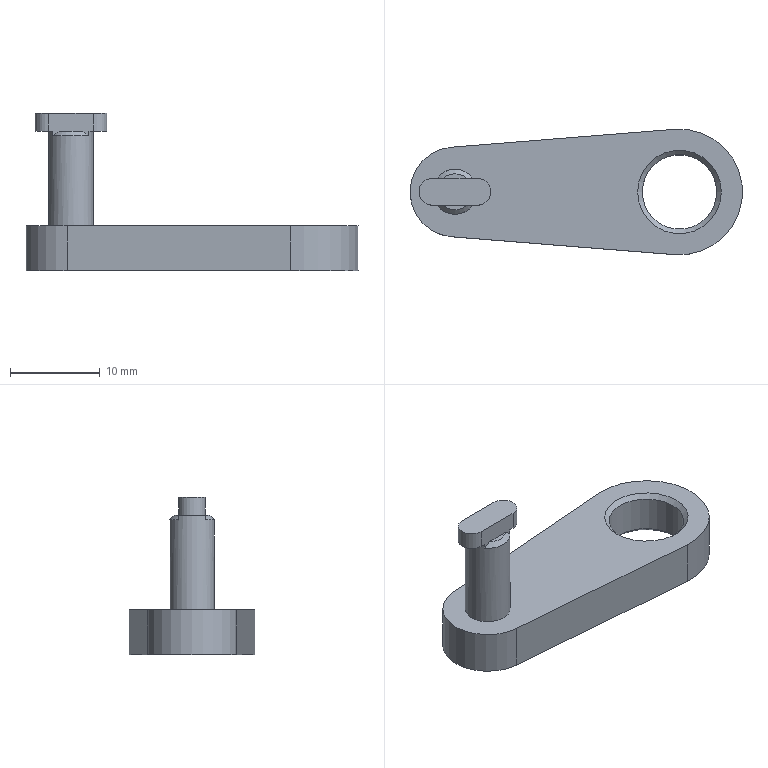Part | NX | features BREP 1 | 1 solid | 21 faces | box 37 x 14 x 17.5 mm | volume 2058 mm3 | plane 11 | cylinder 6 | cone 4 | commonest cylinder face diameters 3 x2 5 x1 8.3 x1 10 x1 14 x1
STEP:
#1=CARTESIAN_POINT('',(4.65,0.,2.5));
#2=VERTEX_POINT('',#1);
#3=CARTESIAN_POINT('',(0.,0.,2.5));
#4=DIRECTION('',(0.,0.,-1.));
#5=DIRECTION('',(1.,0.,0.));
#6=AXIS2_PLACEMENT_3D('',#3,#4,#5);
#7=CIRCLE('',#6,4.65);
#8=EDGE_CURVE('',#2,#2,#7,.T.);
#9=ORIENTED_EDGE('',*,*,#8,.F.);
#10=EDGE_LOOP('',(#9));
#11=FACE_BOUND('',#10,.T.);
#12=CARTESIAN_POINT('',(4.15,0.,2.));
#13=VERTEX_POINT('',#12);
#14=CARTESIAN_POINT('',(0.,0.,2.));
#15=DIRECTION('',(0.,0.,1.));
#16=DIRECTION('',(1.,0.,0.));
#17=AXIS2_PLACEMENT_3D('',#14,#15,#16);
#18=CIRCLE('',#17,4.15);
#19=EDGE_CURVE('',#13,#13,#18,.T.);
#20=ORIENTED_EDGE('',*,*,#19,.F.);
#21=EDGE_LOOP('',(#20));
#22=FACE_BOUND('',#21,.T.);
#23=CARTESIAN_POINT('',(0.,0.,2.));
#24=DIRECTION('',(0.,0.,1.));
#25=DIRECTION('',(-1.,0.,0.));
#26=AXIS2_PLACEMENT_3D('',#23,#24,#25);
#27=CONICAL_SURFACE('',#26,4.15,0.7854);
#28=ADVANCED_FACE('',(#11,#22),#27,.F.);
#29=CARTESIAN_POINT('',(4.65,0.,-2.5));
#30=VERTEX_POINT('',#29);
#31=CARTESIAN_POINT('',(0.,0.,-2.5));
#32=DIRECTION('',(0.,0.,1.));
#33=DIRECTION('',(1.,0.,0.));
#34=AXIS2_PLACEMENT_3D('',#31,#32,#33);
#35=CIRCLE('',#34,4.65);
#36=EDGE_CURVE('',#30,#30,#35,.T.);
#37=ORIENTED_EDGE('',*,*,#36,.F.);
#38=EDGE_LOOP('',(#37));
#39=FACE_BOUND('',#38,.T.);
#40=CARTESIAN_POINT('',(4.15,0.,-2.));
#41=VERTEX_POINT('',#40);
#42=CARTESIAN_POINT('',(0.,0.,-2.));
#43=DIRECTION('',(0.,0.,-1.));
#44=DIRECTION('',(1.,0.,0.));
#45=AXIS2_PLACEMENT_3D('',#42,#43,#44);
#46=CIRCLE('',#45,4.15);
#47=EDGE_CURVE('',#41,#41,#46,.T.);
#48=ORIENTED_EDGE('',*,*,#47,.F.);
#49=EDGE_LOOP('',(#48));
#50=FACE_BOUND('',#49,.T.);
#51=CARTESIAN_POINT('',(0.,0.,-2.5));
#52=DIRECTION('',(0.,0.,-1.));
#53=DIRECTION('',(1.,0.,0.));
#54=AXIS2_PLACEMENT_3D('',#51,#52,#53);
#55=CONICAL_SURFACE('',#54,4.65,0.7854);
#56=ADVANCED_FACE('',(#39,#50),#55,.F.);
#57=ORIENTED_EDGE('',*,*,#19,.T.);
#58=EDGE_LOOP('',(#57));
#59=FACE_BOUND('',#58,.T.);
#60=ORIENTED_EDGE('',*,*,#47,.T.);
#61=EDGE_LOOP('',(#60));
#62=FACE_BOUND('',#61,.T.);
#63=CARTESIAN_POINT('',(0.,0.,-2.5));
#64=DIRECTION('',(0.,0.,1.));
#65=DIRECTION('',(-1.,0.,0.));
#66=AXIS2_PLACEMENT_3D('',#63,#64,#65);
#67=CYLINDRICAL_SURFACE('',#66,4.15);
#68=ADVANCED_FACE('',(#59,#62),#67,.F.);
#69=CARTESIAN_POINT('',(-27.5,1.5,15.));
#70=VERTEX_POINT('',#69);
#71=CARTESIAN_POINT('',(-27.5,-1.5,15.));
#72=VERTEX_POINT('',#71);
#73=CARTESIAN_POINT('',(-27.5,0.,15.));
#74=DIRECTION('',(0.,0.,1.));
#75=DIRECTION('',(1.,0.,0.));
#76=AXIS2_PLACEMENT_3D('',#73,#74,#75);
#77=CIRCLE('',#76,1.5);
#78=EDGE_CURVE('',#70,#72,#77,.T.);
#79=ORIENTED_EDGE('',*,*,#78,.F.);
#80=CARTESIAN_POINT('',(-27.5,1.5,13.));
#81=VERTEX_POINT('',#80);
#82=CARTESIAN_POINT('',(-27.5,1.5,15.));
#83=DIRECTION('',(0.,0.,-1.));
#84=VECTOR('',#83,1000.);
#85=LINE('',#82,#84);
#86=EDGE_CURVE('',#70,#81,#85,.T.);
#87=ORIENTED_EDGE('',*,*,#86,.T.);
#88=CARTESIAN_POINT('',(-27.5,-1.5,13.));
#89=VERTEX_POINT('',#88);
#90=CARTESIAN_POINT('',(-27.5,0.,13.));
#91=DIRECTION('',(0.,0.,1.));
#92=DIRECTION('',(1.,0.,0.));
#93=AXIS2_PLACEMENT_3D('',#90,#91,#92);
#94=CIRCLE('',#93,1.5);
#95=EDGE_CURVE('',#81,#89,#94,.T.);
#96=ORIENTED_EDGE('',*,*,#95,.T.);
#97=CARTESIAN_POINT('',(-27.5,-1.5,15.));
#98=DIRECTION('',(0.,0.,-1.));
#99=VECTOR('',#98,1000.);
#100=LINE('',#97,#99);
#101=EDGE_CURVE('',#72,#89,#100,.T.);
#102=ORIENTED_EDGE('',*,*,#101,.F.);
#103=EDGE_LOOP('',(#79,#87,#96,#102));
#104=FACE_BOUND('',#103,.T.);
#105=CARTESIAN_POINT('',(-27.5,0.,15.));
#106=DIRECTION('',(0.,0.,-1.));
#107=DIRECTION('',(1.,0.,0.));
#108=AXIS2_PLACEMENT_3D('',#105,#106,#107);
#109=CYLINDRICAL_SURFACE('',#108,1.5);
#110=ADVANCED_FACE('',(#104),#109,.T.);
#111=CARTESIAN_POINT('',(-22.5,0.,2.5));
#112=VERTEX_POINT('',#111);
#113=CARTESIAN_POINT('',(-25.,0.,2.5));
#114=DIRECTION('',(0.,0.,1.));
#115=DIRECTION('',(1.,0.,0.));
#116=AXIS2_PLACEMENT_3D('',#113,#114,#115);
#117=CIRCLE('',#116,2.5);
#118=EDGE_CURVE('',#112,#112,#117,.T.);
#119=ORIENTED_EDGE('',*,*,#118,.T.);
#120=EDGE_LOOP('',(#119));
#121=FACE_BOUND('',#120,.T.);
#122=CARTESIAN_POINT('',(-23.,-1.5,13.));
#123=VERTEX_POINT('',#122);
#124=CARTESIAN_POINT('',(-23.,1.5,13.));
#125=VERTEX_POINT('',#124);
#126=CARTESIAN_POINT('',(-25.,0.,13.));
#127=DIRECTION('',(0.,0.,1.));
#128=DIRECTION('',(1.,0.,0.));
#129=AXIS2_PLACEMENT_3D('',#126,#127,#128);
#130=CIRCLE('',#129,2.5);
#131=EDGE_CURVE('',#123,#125,#130,.T.);
#132=ORIENTED_EDGE('',*,*,#131,.F.);
#133=CARTESIAN_POINT('',(-23.,-1.5,12.5));
#134=VERTEX_POINT('',#133);
#135=CARTESIAN_POINT('',(-23.,-1.5,13.));
#136=DIRECTION('',(0.,0.,-1.));
#137=VECTOR('',#136,1000.);
#138=LINE('',#135,#137);
#139=EDGE_CURVE('',#123,#134,#138,.T.);
#140=ORIENTED_EDGE('',*,*,#139,.T.);
#141=CARTESIAN_POINT('',(-27.,-1.5,12.5));
#142=VERTEX_POINT('',#141);
#143=CARTESIAN_POINT('',(-25.,0.,12.5));
#144=DIRECTION('',(0.,0.,-1.));
#145=DIRECTION('',(1.,0.,0.));
#146=AXIS2_PLACEMENT_3D('',#143,#144,#145);
#147=CIRCLE('',#146,2.5);
#148=EDGE_CURVE('',#134,#142,#147,.T.);
#149=ORIENTED_EDGE('',*,*,#148,.T.);
#150=CARTESIAN_POINT('',(-27.,-1.5,13.));
#151=VERTEX_POINT('',#150);
#152=CARTESIAN_POINT('',(-27.,-1.5,12.5));
#153=DIRECTION('',(0.,0.,1.));
#154=VECTOR('',#153,1000.);
#155=LINE('',#152,#154);
#156=EDGE_CURVE('',#142,#151,#155,.T.);
#157=ORIENTED_EDGE('',*,*,#156,.T.);
#158=CARTESIAN_POINT('',(-27.,1.5,13.));
#159=VERTEX_POINT('',#158);
#160=CARTESIAN_POINT('',(-25.,0.,13.));
#161=DIRECTION('',(0.,0.,1.));
#162=DIRECTION('',(1.,0.,0.));
#163=AXIS2_PLACEMENT_3D('',#160,#161,#162);
#164=CIRCLE('',#163,2.5);
#165=EDGE_CURVE('',#159,#151,#164,.T.);
#166=ORIENTED_EDGE('',*,*,#165,.F.);
#167=CARTESIAN_POINT('',(-27.,1.5,12.5));
#168=VERTEX_POINT('',#167);
#169=CARTESIAN_POINT('',(-27.,1.5,13.));
#170=DIRECTION('',(0.,0.,-1.));
#171=VECTOR('',#170,1000.);
#172=LINE('',#169,#171);
#173=EDGE_CURVE('',#159,#168,#172,.T.);
#174=ORIENTED_EDGE('',*,*,#173,.T.);
#175=CARTESIAN_POINT('',(-23.,1.5,12.5));
#176=VERTEX_POINT('',#175);
#177=CARTESIAN_POINT('',(-25.,0.,12.5));
#178=DIRECTION('',(0.,0.,-1.));
#179=DIRECTION('',(1.,0.,0.));
#180=AXIS2_PLACEMENT_3D('',#177,#178,#179);
#181=CIRCLE('',#180,2.5);
#182=EDGE_CURVE('',#168,#176,#181,.T.);
#183=ORIENTED_EDGE('',*,*,#182,.T.);
#184=CARTESIAN_POINT('',(-23.,1.5,12.5));
#185=DIRECTION('',(0.,0.,1.));
#186=VECTOR('',#185,1000.);
#187=LINE('',#184,#186);
#188=EDGE_CURVE('',#176,#125,#187,.T.);
#189=ORIENTED_EDGE('',*,*,#188,.T.);
#190=EDGE_LOOP('',(#132,#140,#149,#157,#166,#174,#183,#189));
#191=FACE_BOUND('',#190,.T.);
#192=CARTESIAN_POINT('',(-25.,0.,13.));
#193=DIRECTION('',(0.,0.,-1.));
#194=DIRECTION('',(1.,0.,0.));
#195=AXIS2_PLACEMENT_3D('',#192,#193,#194);
#196=CYLINDRICAL_SURFACE('',#195,2.5);
#197=ADVANCED_FACE('',(#121,#191),#196,.T.);
#198=CARTESIAN_POINT('',(-25.4,4.984,2.5));
#199=VERTEX_POINT('',#198);
#200=CARTESIAN_POINT('',(-25.4,-4.984,2.5));
#201=VERTEX_POINT('',#200);
#202=CARTESIAN_POINT('',(-25.,0.,2.5));
#203=DIRECTION('',(0.,0.,1.));
#204=DIRECTION('',(1.,0.,0.));
#205=AXIS2_PLACEMENT_3D('',#202,#203,#204);
#206=CIRCLE('',#205,5.);
#207=EDGE_CURVE('',#199,#201,#206,.T.);
#208=ORIENTED_EDGE('',*,*,#207,.F.);
#209=CARTESIAN_POINT('',(-25.4,4.984,-2.5));
#210=VERTEX_POINT('',#209);
#211=CARTESIAN_POINT('',(-25.4,4.984,2.5));
#212=DIRECTION('',(0.,0.,-1.));
#213=VECTOR('',#212,1000.);
#214=LINE('',#211,#213);
#215=EDGE_CURVE('',#199,#210,#214,.T.);
#216=ORIENTED_EDGE('',*,*,#215,.T.);
#217=CARTESIAN_POINT('',(-25.4,-4.984,-2.5));
#218=VERTEX_POINT('',#217);
#219=CARTESIAN_POINT('',(-25.,0.,-2.5));
#220=DIRECTION('',(0.,0.,1.));
#221=DIRECTION('',(1.,0.,0.));
#222=AXIS2_PLACEMENT_3D('',#219,#220,#221);
#223=CIRCLE('',#222,5.);
#224=EDGE_CURVE('',#210,#218,#223,.T.);
#225=ORIENTED_EDGE('',*,*,#224,.T.);
#226=CARTESIAN_POINT('',(-25.4,-4.984,2.5));
#227=DIRECTION('',(0.,0.,-1.));
#228=VECTOR('',#227,1000.);
#229=LINE('',#226,#228);
#230=EDGE_CURVE('',#201,#218,#229,.T.);
#231=ORIENTED_EDGE('',*,*,#230,.F.);
#232=EDGE_LOOP('',(#208,#216,#225,#231));
#233=FACE_BOUND('',#232,.T.);
#234=CARTESIAN_POINT('',(-25.,0.,2.5));
#235=DIRECTION('',(0.,0.,-1.));
#236=DIRECTION('',(1.,0.,0.));
#237=AXIS2_PLACEMENT_3D('',#234,#235,#236);
#238=CYLINDRICAL_SURFACE('',#237,5.);
#239=ADVANCED_FACE('',(#233),#238,.T.);
#240=CARTESIAN_POINT('',(-23.677,1.5,13.));
#241=VERTEX_POINT('',#240);
#242=CARTESIAN_POINT('',(-26.323,1.5,13.));
#243=VERTEX_POINT('',#242);
#244=CARTESIAN_POINT('',(-27.5,1.5,13.));
#245=DIRECTION('',(-1.,0.,0.));
#246=VECTOR('',#245,1000.);
#247=LINE('',#244,#246);
#248=EDGE_CURVE('',#241,#243,#247,.T.);
#249=ORIENTED_EDGE('',*,*,#248,.F.);
#250=CARTESIAN_POINT('',(-25.,0.,13.));
#251=DIRECTION('',(0.,0.,1.));
#252=DIRECTION('',(1.,0.,0.));
#253=AXIS2_PLACEMENT_3D('',#250,#251,#252);
#254=CIRCLE('',#253,2.);
#255=EDGE_CURVE('',#241,#243,#254,.T.);
#256=ORIENTED_EDGE('',*,*,#255,.T.);
#257=EDGE_LOOP('',(#249,#256));
#258=FACE_BOUND('',#257,.T.);
#259=CARTESIAN_POINT('',(-25.,0.,13.));
#260=DIRECTION('',(0.,0.,1.));
#261=DIRECTION('',(-1.,0.,0.));
#262=AXIS2_PLACEMENT_3D('',#259,#260,#261);
#263=PLANE('',#262);
#264=ADVANCED_FACE('',(#258),#263,.T.);
#265=ORIENTED_EDGE('',*,*,#8,.T.);
#266=EDGE_LOOP('',(#265));
#267=FACE_BOUND('',#266,.T.);
#268=CARTESIAN_POINT('',(-0.56,6.978,2.5));
#269=VERTEX_POINT('',#268);
#270=CARTESIAN_POINT('',(-25.4,4.984,2.5));
#271=DIRECTION('',(-0.9968,-0.08,0.));
#272=VECTOR('',#271,1000.);
#273=LINE('',#270,#272);
#274=EDGE_CURVE('',#269,#199,#273,.T.);
#275=ORIENTED_EDGE('',*,*,#274,.T.);
#276=ORIENTED_EDGE('',*,*,#207,.T.);
#277=CARTESIAN_POINT('',(-0.56,-6.978,2.5));
#278=VERTEX_POINT('',#277);
#279=CARTESIAN_POINT('',(-0.56,-6.978,2.5));
#280=DIRECTION('',(0.9968,-0.08,0.));
#281=VECTOR('',#280,1000.);
#282=LINE('',#279,#281);
#283=EDGE_CURVE('',#201,#278,#282,.T.);
#284=ORIENTED_EDGE('',*,*,#283,.T.);
#285=CARTESIAN_POINT('',(0.,0.,2.5));
#286=DIRECTION('',(0.,0.,1.));
#287=DIRECTION('',(1.,0.,0.));
#288=AXIS2_PLACEMENT_3D('',#285,#286,#287);
#289=CIRCLE('',#288,7.);
#290=EDGE_CURVE('',#278,#269,#289,.T.);
#291=ORIENTED_EDGE('',*,*,#290,.T.);
#292=EDGE_LOOP('',(#275,#276,#284,#291));
#293=FACE_BOUND('',#292,.T.);
#294=ORIENTED_EDGE('',*,*,#118,.F.);
#295=EDGE_LOOP('',(#294));
#296=FACE_BOUND('',#295,.T.);
#297=CARTESIAN_POINT('',(-25.,0.,2.5));
#298=DIRECTION('',(0.,0.,1.));
#299=DIRECTION('',(-1.,0.,0.));
#300=AXIS2_PLACEMENT_3D('',#297,#298,#299);
#301=PLANE('',#300);
#302=ADVANCED_FACE('',(#267,#293,#296),#301,.T.);
#303=CARTESIAN_POINT('',(-0.56,-6.978,-2.5));
#304=VERTEX_POINT('',#303);
#305=CARTESIAN_POINT('',(-0.56,-6.978,-2.5));
#306=DIRECTION('',(0.9968,-0.08,0.));
#307=VECTOR('',#306,1000.);
#308=LINE('',#305,#307);
#309=EDGE_CURVE('',#218,#304,#308,.T.);
#310=ORIENTED_EDGE('',*,*,#309,.T.);
#311=CARTESIAN_POINT('',(-0.56,-6.978,2.5));
#312=DIRECTION('',(0.,0.,-1.));
#313=VECTOR('',#312,1000.);
#314=LINE('',#311,#313);
#315=EDGE_CURVE('',#278,#304,#314,.T.);
#316=ORIENTED_EDGE('',*,*,#315,.F.);
#317=ORIENTED_EDGE('',*,*,#283,.F.);
#318=ORIENTED_EDGE('',*,*,#230,.T.);
#319=EDGE_LOOP('',(#310,#316,#317,#318));
#320=FACE_BOUND('',#319,.T.);
#321=CARTESIAN_POINT('',(-0.56,-6.978,2.5));
#322=DIRECTION('',(0.08,0.9968,0.));
#323=DIRECTION('',(0.9968,-0.08,0.));
#324=AXIS2_PLACEMENT_3D('',#321,#322,#323);
#325=PLANE('',#324);
#326=ADVANCED_FACE('',(#320),#325,.F.);
#327=CARTESIAN_POINT('',(-0.56,6.978,-2.5));
#328=VERTEX_POINT('',#327);
#329=CARTESIAN_POINT('',(0.,0.,-2.5));
#330=DIRECTION('',(0.,0.,1.));
#331=DIRECTION('',(1.,0.,0.));
#332=AXIS2_PLACEMENT_3D('',#329,#330,#331);
#333=CIRCLE('',#332,7.);
#334=EDGE_CURVE('',#304,#328,#333,.T.);
#335=ORIENTED_EDGE('',*,*,#334,.T.);
#336=CARTESIAN_POINT('',(-0.56,6.978,2.5));
#337=DIRECTION('',(0.,0.,-1.));
#338=VECTOR('',#337,1000.);
#339=LINE('',#336,#338);
#340=EDGE_CURVE('',#269,#328,#339,.T.);
#341=ORIENTED_EDGE('',*,*,#340,.F.);
#342=ORIENTED_EDGE('',*,*,#290,.F.);
#343=ORIENTED_EDGE('',*,*,#315,.T.);
#344=EDGE_LOOP('',(#335,#341,#342,#343));
#345=FACE_BOUND('',#344,.T.);
#346=CARTESIAN_POINT('',(0.,0.,2.5));
#347=DIRECTION('',(0.,0.,-1.));
#348=DIRECTION('',(1.,0.,0.));
#349=AXIS2_PLACEMENT_3D('',#346,#347,#348);
#350=CYLINDRICAL_SURFACE('',#349,7.);
#351=ADVANCED_FACE('',(#345),#350,.T.);
#352=CARTESIAN_POINT('',(-25.4,4.984,-2.5));
#353=DIRECTION('',(-0.9968,-0.08,0.));
#354=VECTOR('',#353,1000.);
#355=LINE('',#352,#354);
#356=EDGE_CURVE('',#328,#210,#355,.T.);
#357=ORIENTED_EDGE('',*,*,#356,.T.);
#358=ORIENTED_EDGE('',*,*,#215,.F.);
#359=ORIENTED_EDGE('',*,*,#274,.F.);
#360=ORIENTED_EDGE('',*,*,#340,.T.);
#361=EDGE_LOOP('',(#357,#358,#359,#360));
#362=FACE_BOUND('',#361,.T.);
#363=CARTESIAN_POINT('',(-25.4,4.984,2.5));
#364=DIRECTION('',(0.08,-0.9968,0.));
#365=DIRECTION('',(-0.9968,-0.08,0.));
#366=AXIS2_PLACEMENT_3D('',#363,#364,#365);
#367=PLANE('',#366);
#368=ADVANCED_FACE('',(#362),#367,.F.);
#369=ORIENTED_EDGE('',*,*,#36,.T.);
#370=EDGE_LOOP('',(#369));
#371=FACE_BOUND('',#370,.T.);
#372=ORIENTED_EDGE('',*,*,#224,.F.);
#373=ORIENTED_EDGE('',*,*,#356,.F.);
#374=ORIENTED_EDGE('',*,*,#334,.F.);
#375=ORIENTED_EDGE('',*,*,#309,.F.);
#376=EDGE_LOOP('',(#372,#373,#374,#375));
#377=FACE_BOUND('',#376,.T.);
#378=CARTESIAN_POINT('',(-25.,0.,-2.5));
#379=DIRECTION('',(0.,0.,1.));
#380=DIRECTION('',(-1.,0.,0.));
#381=AXIS2_PLACEMENT_3D('',#378,#379,#380);
#382=PLANE('',#381);
#383=ADVANCED_FACE('',(#371,#377),#382,.F.);
#384=CARTESIAN_POINT('',(-26.323,-1.5,13.));
#385=VERTEX_POINT('',#384);
#386=CARTESIAN_POINT('',(-23.677,-1.5,13.));
#387=VERTEX_POINT('',#386);
#388=CARTESIAN_POINT('',(-27.5,-1.5,13.));
#389=DIRECTION('',(1.,0.,0.));
#390=VECTOR('',#389,1000.);
#391=LINE('',#388,#390);
#392=EDGE_CURVE('',#385,#387,#391,.T.);
#393=ORIENTED_EDGE('',*,*,#392,.F.);
#394=CARTESIAN_POINT('',(-25.,0.,13.));
#395=DIRECTION('',(0.,0.,1.));
#396=DIRECTION('',(1.,0.,0.));
#397=AXIS2_PLACEMENT_3D('',#394,#395,#396);
#398=CIRCLE('',#397,2.);
#399=EDGE_CURVE('',#385,#387,#398,.T.);
#400=ORIENTED_EDGE('',*,*,#399,.T.);
#401=EDGE_LOOP('',(#393,#400));
#402=FACE_BOUND('',#401,.T.);
#403=CARTESIAN_POINT('',(-25.,0.,13.));
#404=DIRECTION('',(0.,0.,1.));
#405=DIRECTION('',(-1.,0.,0.));
#406=AXIS2_PLACEMENT_3D('',#403,#404,#405);
#407=PLANE('',#406);
#408=ADVANCED_FACE('',(#402),#407,.T.);
#409=CARTESIAN_POINT('',(-27.5,1.5,13.));
#410=DIRECTION('',(-1.,0.,0.));
#411=VECTOR('',#410,1000.);
#412=LINE('',#409,#411);
#413=EDGE_CURVE('',#159,#81,#412,.T.);
#414=ORIENTED_EDGE('',*,*,#413,.F.);
#415=ORIENTED_EDGE('',*,*,#165,.T.);
#416=CARTESIAN_POINT('',(-27.5,-1.5,13.));
#417=DIRECTION('',(1.,0.,0.));
#418=VECTOR('',#417,1000.);
#419=LINE('',#416,#418);
#420=EDGE_CURVE('',#89,#151,#419,.T.);
#421=ORIENTED_EDGE('',*,*,#420,.F.);
#422=ORIENTED_EDGE('',*,*,#95,.F.);
#423=EDGE_LOOP('',(#414,#415,#421,#422));
#424=FACE_BOUND('',#423,.T.);
#425=CARTESIAN_POINT('',(-27.5,0.,13.));
#426=DIRECTION('',(0.,0.,1.));
#427=DIRECTION('',(-1.,0.,0.));
#428=AXIS2_PLACEMENT_3D('',#425,#426,#427);
#429=PLANE('',#428);
#430=ADVANCED_FACE('',(#424),#429,.F.);
#431=CARTESIAN_POINT('',(-22.5,-1.5,13.));
#432=VERTEX_POINT('',#431);
#433=CARTESIAN_POINT('',(-27.5,-1.5,13.));
#434=DIRECTION('',(1.,0.,0.));
#435=VECTOR('',#434,1000.);
#436=LINE('',#433,#435);
#437=EDGE_CURVE('',#123,#432,#436,.T.);
#438=ORIENTED_EDGE('',*,*,#437,.F.);
#439=ORIENTED_EDGE('',*,*,#131,.T.);
#440=CARTESIAN_POINT('',(-22.5,1.5,13.));
#441=VERTEX_POINT('',#440);
#442=CARTESIAN_POINT('',(-27.5,1.5,13.));
#443=DIRECTION('',(-1.,0.,0.));
#444=VECTOR('',#443,1000.);
#445=LINE('',#442,#444);
#446=EDGE_CURVE('',#441,#125,#445,.T.);
#447=ORIENTED_EDGE('',*,*,#446,.F.);
#448=CARTESIAN_POINT('',(-22.5,0.,13.));
#449=DIRECTION('',(0.,0.,1.));
#450=DIRECTION('',(1.,0.,0.));
#451=AXIS2_PLACEMENT_3D('',#448,#449,#450);
#452=CIRCLE('',#451,1.5);
#453=EDGE_CURVE('',#432,#441,#452,.T.);
#454=ORIENTED_EDGE('',*,*,#453,.F.);
#455=EDGE_LOOP('',(#438,#439,#447,#454));
#456=FACE_BOUND('',#455,.T.);
#457=CARTESIAN_POINT('',(-27.5,0.,13.));
#458=DIRECTION('',(0.,0.,1.));
#459=DIRECTION('',(-1.,0.,0.));
#460=AXIS2_PLACEMENT_3D('',#457,#458,#459);
#461=PLANE('',#460);
#462=ADVANCED_FACE('',(#456),#461,.F.);
#463=ORIENTED_EDGE('',*,*,#420,.T.);
#464=ORIENTED_EDGE('',*,*,#156,.F.);
#465=CARTESIAN_POINT('',(-27.,-1.5,12.5));
#466=CARTESIAN_POINT('',(-26.781,-1.5,12.675));
#467=CARTESIAN_POINT('',(-26.557,-1.5,12.845));
#468=CARTESIAN_POINT('',(-26.323,-1.5,13.));
#469=B_SPLINE_CURVE_WITH_KNOTS('',3,(#465,#466,#467,#468),.UNSPECIFIED.,.F.,.F.,(4,4),(0.,0.0008417),.UNSPECIFIED.);
#470=EDGE_CURVE('',#142,#385,#469,.T.);
#471=ORIENTED_EDGE('',*,*,#470,.T.);
#472=ORIENTED_EDGE('',*,*,#392,.T.);
#473=CARTESIAN_POINT('',(-23.677,-1.5,13.));
#474=CARTESIAN_POINT('',(-23.443,-1.5,12.845));
#475=CARTESIAN_POINT('',(-23.219,-1.5,12.675));
#476=CARTESIAN_POINT('',(-23.,-1.5,12.5));
#477=B_SPLINE_CURVE_WITH_KNOTS('',3,(#473,#474,#475,#476),.UNSPECIFIED.,.F.,.F.,(4,4),(0.,0.0008417),.UNSPECIFIED.);
#478=EDGE_CURVE('',#387,#134,#477,.T.);
#479=ORIENTED_EDGE('',*,*,#478,.T.);
#480=ORIENTED_EDGE('',*,*,#139,.F.);
#481=ORIENTED_EDGE('',*,*,#437,.T.);
#482=CARTESIAN_POINT('',(-22.5,-1.5,15.));
#483=VERTEX_POINT('',#482);
#484=CARTESIAN_POINT('',(-22.5,-1.5,15.));
#485=DIRECTION('',(0.,0.,-1.));
#486=VECTOR('',#485,1000.);
#487=LINE('',#484,#486);
#488=EDGE_CURVE('',#483,#432,#487,.T.);
#489=ORIENTED_EDGE('',*,*,#488,.F.);
#490=CARTESIAN_POINT('',(-27.5,-1.5,15.));
#491=DIRECTION('',(1.,0.,0.));
#492=VECTOR('',#491,1000.);
#493=LINE('',#490,#492);
#494=EDGE_CURVE('',#72,#483,#493,.T.);
#495=ORIENTED_EDGE('',*,*,#494,.F.);
#496=ORIENTED_EDGE('',*,*,#101,.T.);
#497=EDGE_LOOP('',(#463,#464,#471,#472,#479,#480,#481,#489,#495,#496));
#498=FACE_BOUND('',#497,.T.);
#499=CARTESIAN_POINT('',(-27.5,-1.5,15.));
#500=DIRECTION('',(0.,1.,0.));
#501=DIRECTION('',(1.,0.,0.));
#502=AXIS2_PLACEMENT_3D('',#499,#500,#501);
#503=PLANE('',#502);
#504=ADVANCED_FACE('',(#498),#503,.F.);
#505=ORIENTED_EDGE('',*,*,#453,.T.);
#506=CARTESIAN_POINT('',(-22.5,1.5,15.));
#507=VERTEX_POINT('',#506);
#508=CARTESIAN_POINT('',(-22.5,1.5,15.));
#509=DIRECTION('',(0.,0.,-1.));
#510=VECTOR('',#509,1000.);
#511=LINE('',#508,#510);
#512=EDGE_CURVE('',#507,#441,#511,.T.);
#513=ORIENTED_EDGE('',*,*,#512,.F.);
#514=CARTESIAN_POINT('',(-22.5,0.,15.));
#515=DIRECTION('',(0.,0.,1.));
#516=DIRECTION('',(1.,0.,0.));
#517=AXIS2_PLACEMENT_3D('',#514,#515,#516);
#518=CIRCLE('',#517,1.5);
#519=EDGE_CURVE('',#483,#507,#518,.T.);
#520=ORIENTED_EDGE('',*,*,#519,.F.);
#521=ORIENTED_EDGE('',*,*,#488,.T.);
#522=EDGE_LOOP('',(#505,#513,#520,#521));
#523=FACE_BOUND('',#522,.T.);
#524=CARTESIAN_POINT('',(-22.5,0.,15.));
#525=DIRECTION('',(0.,0.,-1.));
#526=DIRECTION('',(1.,0.,0.));
#527=AXIS2_PLACEMENT_3D('',#524,#525,#526);
#528=CYLINDRICAL_SURFACE('',#527,1.5);
#529=ADVANCED_FACE('',(#523),#528,.T.);
#530=ORIENTED_EDGE('',*,*,#446,.T.);
#531=ORIENTED_EDGE('',*,*,#188,.F.);
#532=CARTESIAN_POINT('',(-23.,1.5,12.5));
#533=CARTESIAN_POINT('',(-23.219,1.5,12.675));
#534=CARTESIAN_POINT('',(-23.443,1.5,12.845));
#535=CARTESIAN_POINT('',(-23.677,1.5,13.));
#536=B_SPLINE_CURVE_WITH_KNOTS('',3,(#532,#533,#534,#535),.UNSPECIFIED.,.F.,.F.,(4,4),(0.,0.0008417),.UNSPECIFIED.);
#537=EDGE_CURVE('',#176,#241,#536,.T.);
#538=ORIENTED_EDGE('',*,*,#537,.T.);
#539=ORIENTED_EDGE('',*,*,#248,.T.);
#540=CARTESIAN_POINT('',(-26.323,1.5,13.));
#541=CARTESIAN_POINT('',(-26.557,1.5,12.845));
#542=CARTESIAN_POINT('',(-26.781,1.5,12.675));
#543=CARTESIAN_POINT('',(-27.,1.5,12.5));
#544=B_SPLINE_CURVE_WITH_KNOTS('',3,(#540,#541,#542,#543),.UNSPECIFIED.,.F.,.F.,(4,4),(0.,0.0008417),.UNSPECIFIED.);
#545=EDGE_CURVE('',#243,#168,#544,.T.);
#546=ORIENTED_EDGE('',*,*,#545,.T.);
#547=ORIENTED_EDGE('',*,*,#173,.F.);
#548=ORIENTED_EDGE('',*,*,#413,.T.);
#549=ORIENTED_EDGE('',*,*,#86,.F.);
#550=CARTESIAN_POINT('',(-27.5,1.5,15.));
#551=DIRECTION('',(-1.,0.,0.));
#552=VECTOR('',#551,1000.);
#553=LINE('',#550,#552);
#554=EDGE_CURVE('',#507,#70,#553,.T.);
#555=ORIENTED_EDGE('',*,*,#554,.F.);
#556=ORIENTED_EDGE('',*,*,#512,.T.);
#557=EDGE_LOOP('',(#530,#531,#538,#539,#546,#547,#548,#549,#555,#556));
#558=FACE_BOUND('',#557,.T.);
#559=CARTESIAN_POINT('',(-27.5,1.5,15.));
#560=DIRECTION('',(0.,-1.,0.));
#561=DIRECTION('',(-1.,0.,0.));
#562=AXIS2_PLACEMENT_3D('',#559,#560,#561);
#563=PLANE('',#562);
#564=ADVANCED_FACE('',(#558),#563,.F.);
#565=ORIENTED_EDGE('',*,*,#554,.T.);
#566=ORIENTED_EDGE('',*,*,#78,.T.);
#567=ORIENTED_EDGE('',*,*,#494,.T.);
#568=ORIENTED_EDGE('',*,*,#519,.T.);
#569=EDGE_LOOP('',(#565,#566,#567,#568));
#570=FACE_BOUND('',#569,.T.);
#571=CARTESIAN_POINT('',(-27.5,0.,15.));
#572=DIRECTION('',(0.,0.,1.));
#573=DIRECTION('',(-1.,0.,0.));
#574=AXIS2_PLACEMENT_3D('',#571,#572,#573);
#575=PLANE('',#574);
#576=ADVANCED_FACE('',(#570),#575,.T.);
#577=ORIENTED_EDGE('',*,*,#537,.F.);
#578=ORIENTED_EDGE('',*,*,#182,.F.);
#579=ORIENTED_EDGE('',*,*,#545,.F.);
#580=ORIENTED_EDGE('',*,*,#255,.F.);
#581=EDGE_LOOP('',(#577,#578,#579,#580));
#582=FACE_BOUND('',#581,.T.);
#583=CARTESIAN_POINT('',(-25.,0.,13.));
#584=DIRECTION('',(0.,0.,-1.));
#585=DIRECTION('',(1.,0.,0.));
#586=AXIS2_PLACEMENT_3D('',#583,#584,#585);
#587=CONICAL_SURFACE('',#586,2.,0.7854);
#588=ADVANCED_FACE('',(#582),#587,.T.);
#589=ORIENTED_EDGE('',*,*,#470,.F.);
#590=ORIENTED_EDGE('',*,*,#148,.F.);
#591=ORIENTED_EDGE('',*,*,#478,.F.);
#592=ORIENTED_EDGE('',*,*,#399,.F.);
#593=EDGE_LOOP('',(#589,#590,#591,#592));
#594=FACE_BOUND('',#593,.T.);
#595=CARTESIAN_POINT('',(-25.,0.,13.));
#596=DIRECTION('',(0.,0.,-1.));
#597=DIRECTION('',(1.,0.,0.));
#598=AXIS2_PLACEMENT_3D('',#595,#596,#597);
#599=CONICAL_SURFACE('',#598,2.,0.7854);
#600=ADVANCED_FACE('',(#594),#599,.T.);
#601=CLOSED_SHELL('',(#28,#56,#68,#110,#197,#239,#264,#302,#326,#351,#368,#383,#408,#430,#462,#504,#529,#564,#576,#588,#600));
#602=MANIFOLD_SOLID_BREP('',#601);
#603=(LENGTH_UNIT()NAMED_UNIT(*)SI_UNIT(.MILLI.,.METRE.));
#604=UNCERTAINTY_MEASURE_WITH_UNIT(LENGTH_MEASURE(0.0508),#603,'','');
#605=(NAMED_UNIT(*)PLANE_ANGLE_UNIT()SI_UNIT($,.RADIAN.));
#606=(NAMED_UNIT(*)SI_UNIT($,.STERADIAN.)SOLID_ANGLE_UNIT());
#607=(GEOMETRIC_REPRESENTATION_CONTEXT(3)GLOBAL_UNCERTAINTY_ASSIGNED_CONTEXT((#604))GLOBAL_UNIT_ASSIGNED_CONTEXT((#603,#605,#606))REPRESENTATION_CONTEXT('',''));
#608=ADVANCED_BREP_SHAPE_REPRESENTATION('',(#602),#607);